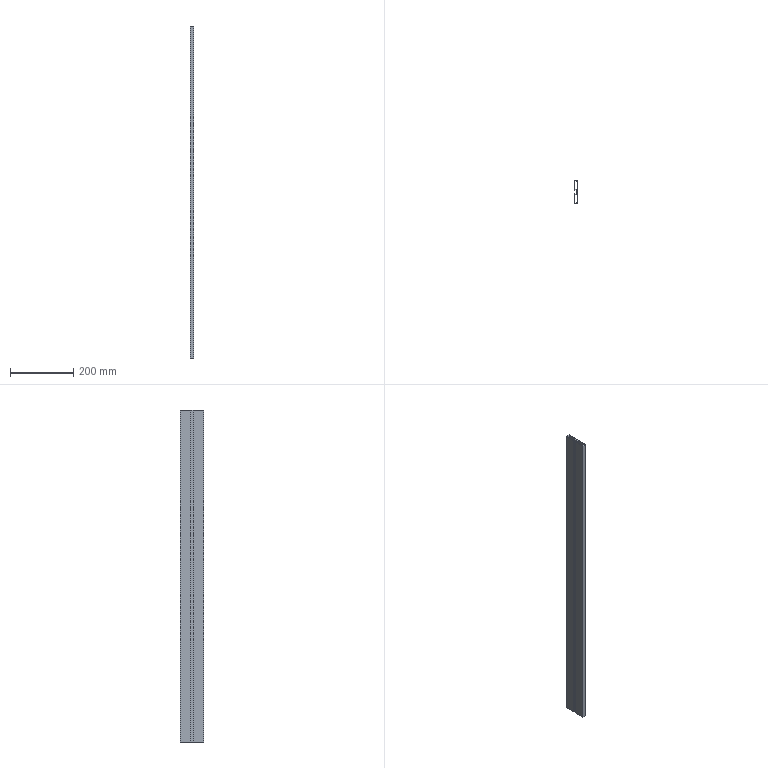Part | SolidWorks | features Extrusion 1 | 1 solid | 22 faces | box 12 x 73 x 1050 mm | volume 382200 mm3 | plane 22
STEP:
#1=CARTESIAN_POINT('',(-12.,36.5,525.));
#2=VERTEX_POINT('',#1);
#3=CARTESIAN_POINT('',(-12.,4.5,525.));
#4=VERTEX_POINT('',#3);
#5=CARTESIAN_POINT('',(-12.,36.5,525.));
#6=DIRECTION('',(0.,-1.,0.));
#7=VECTOR('',#6,1000.);
#8=LINE('',#5,#7);
#9=EDGE_CURVE('',#2,#4,#8,.T.);
#10=ORIENTED_EDGE('',*,*,#9,.T.);
#11=CARTESIAN_POINT('',(-10.,4.5,525.));
#12=VERTEX_POINT('',#11);
#13=CARTESIAN_POINT('',(-12.,4.5,525.));
#14=DIRECTION('',(1.,0.,0.));
#15=VECTOR('',#14,1000.);
#16=LINE('',#13,#15);
#17=EDGE_CURVE('',#4,#12,#16,.T.);
#18=ORIENTED_EDGE('',*,*,#17,.T.);
#19=CARTESIAN_POINT('',(-10.,6.5,525.));
#20=VERTEX_POINT('',#19);
#21=CARTESIAN_POINT('',(-10.,4.5,525.));
#22=DIRECTION('',(0.,1.,0.));
#23=VECTOR('',#22,1000.);
#24=LINE('',#21,#23);
#25=EDGE_CURVE('',#12,#20,#24,.T.);
#26=ORIENTED_EDGE('',*,*,#25,.T.);
#27=CARTESIAN_POINT('',(-4.,6.5,525.));
#28=VERTEX_POINT('',#27);
#29=CARTESIAN_POINT('',(-10.,6.5,525.));
#30=DIRECTION('',(1.,0.,0.));
#31=VECTOR('',#30,1000.);
#32=LINE('',#29,#31);
#33=EDGE_CURVE('',#20,#28,#32,.T.);
#34=ORIENTED_EDGE('',*,*,#33,.T.);
#35=CARTESIAN_POINT('',(-4.,-6.5,525.));
#36=VERTEX_POINT('',#35);
#37=CARTESIAN_POINT('',(-4.,6.5,525.));
#38=DIRECTION('',(0.,-1.,0.));
#39=VECTOR('',#38,1000.);
#40=LINE('',#37,#39);
#41=EDGE_CURVE('',#28,#36,#40,.T.);
#42=ORIENTED_EDGE('',*,*,#41,.T.);
#43=CARTESIAN_POINT('',(-10.,-6.5,525.));
#44=VERTEX_POINT('',#43);
#45=CARTESIAN_POINT('',(-4.,-6.5,525.));
#46=DIRECTION('',(-1.,0.,0.));
#47=VECTOR('',#46,1000.);
#48=LINE('',#45,#47);
#49=EDGE_CURVE('',#36,#44,#48,.T.);
#50=ORIENTED_EDGE('',*,*,#49,.T.);
#51=CARTESIAN_POINT('',(-10.,-4.5,525.));
#52=VERTEX_POINT('',#51);
#53=CARTESIAN_POINT('',(-10.,-6.5,525.));
#54=DIRECTION('',(0.,1.,0.));
#55=VECTOR('',#54,1000.);
#56=LINE('',#53,#55);
#57=EDGE_CURVE('',#44,#52,#56,.T.);
#58=ORIENTED_EDGE('',*,*,#57,.T.);
#59=CARTESIAN_POINT('',(-12.,-4.5,525.));
#60=VERTEX_POINT('',#59);
#61=CARTESIAN_POINT('',(-10.,-4.5,525.));
#62=DIRECTION('',(-1.,0.,0.));
#63=VECTOR('',#62,1000.);
#64=LINE('',#61,#63);
#65=EDGE_CURVE('',#52,#60,#64,.T.);
#66=ORIENTED_EDGE('',*,*,#65,.T.);
#67=CARTESIAN_POINT('',(-12.,-36.5,525.));
#68=VERTEX_POINT('',#67);
#69=CARTESIAN_POINT('',(-12.,-4.5,525.));
#70=DIRECTION('',(0.,-1.,0.));
#71=VECTOR('',#70,1000.);
#72=LINE('',#69,#71);
#73=EDGE_CURVE('',#60,#68,#72,.T.);
#74=ORIENTED_EDGE('',*,*,#73,.T.);
#75=CARTESIAN_POINT('',(0.,-36.5,525.));
#76=VERTEX_POINT('',#75);
#77=CARTESIAN_POINT('',(-12.,-36.5,525.));
#78=DIRECTION('',(1.,0.,0.));
#79=VECTOR('',#78,1000.);
#80=LINE('',#77,#79);
#81=EDGE_CURVE('',#68,#76,#80,.T.);
#82=ORIENTED_EDGE('',*,*,#81,.T.);
#83=CARTESIAN_POINT('',(0.,36.5,525.));
#84=VERTEX_POINT('',#83);
#85=CARTESIAN_POINT('',(0.,-36.5,525.));
#86=DIRECTION('',(0.,1.,0.));
#87=VECTOR('',#86,1000.);
#88=LINE('',#85,#87);
#89=EDGE_CURVE('',#76,#84,#88,.T.);
#90=ORIENTED_EDGE('',*,*,#89,.T.);
#91=CARTESIAN_POINT('',(0.,36.5,525.));
#92=DIRECTION('',(-1.,0.,0.));
#93=VECTOR('',#92,1000.);
#94=LINE('',#91,#93);
#95=EDGE_CURVE('',#84,#2,#94,.T.);
#96=ORIENTED_EDGE('',*,*,#95,.T.);
#97=EDGE_LOOP('',(#10,#18,#26,#34,#42,#50,#58,#66,#74,#82,#90,#96));
#98=FACE_OUTER_BOUND('',#97,.T.);
#99=CARTESIAN_POINT('',(-10.,-34.5,525.));
#100=VERTEX_POINT('',#99);
#101=CARTESIAN_POINT('',(-2.,-34.5,525.));
#102=VERTEX_POINT('',#101);
#103=CARTESIAN_POINT('',(-2.,-34.5,525.));
#104=DIRECTION('',(1.,0.,0.));
#105=VECTOR('',#104,1000.);
#106=LINE('',#103,#105);
#107=EDGE_CURVE('',#100,#102,#106,.T.);
#108=ORIENTED_EDGE('',*,*,#107,.F.);
#109=CARTESIAN_POINT('',(-10.,-8.5,525.));
#110=VERTEX_POINT('',#109);
#111=CARTESIAN_POINT('',(-10.,-34.5,525.));
#112=DIRECTION('',(0.,-1.,0.));
#113=VECTOR('',#112,1000.);
#114=LINE('',#111,#113);
#115=EDGE_CURVE('',#110,#100,#114,.T.);
#116=ORIENTED_EDGE('',*,*,#115,.F.);
#117=CARTESIAN_POINT('',(-2.,-8.5,525.));
#118=VERTEX_POINT('',#117);
#119=CARTESIAN_POINT('',(-10.,-8.5,525.));
#120=DIRECTION('',(-1.,0.,0.));
#121=VECTOR('',#120,1000.);
#122=LINE('',#119,#121);
#123=EDGE_CURVE('',#118,#110,#122,.T.);
#124=ORIENTED_EDGE('',*,*,#123,.F.);
#125=CARTESIAN_POINT('',(-2.,-8.5,525.));
#126=DIRECTION('',(0.,1.,0.));
#127=VECTOR('',#126,1000.);
#128=LINE('',#125,#127);
#129=EDGE_CURVE('',#102,#118,#128,.T.);
#130=ORIENTED_EDGE('',*,*,#129,.F.);
#131=EDGE_LOOP('',(#108,#116,#124,#130));
#132=FACE_BOUND('',#131,.T.);
#133=CARTESIAN_POINT('',(-10.,34.5,525.));
#134=VERTEX_POINT('',#133);
#135=CARTESIAN_POINT('',(-10.,8.5,525.));
#136=VERTEX_POINT('',#135);
#137=CARTESIAN_POINT('',(-10.,8.5,525.));
#138=DIRECTION('',(0.,-1.,0.));
#139=VECTOR('',#138,1000.);
#140=LINE('',#137,#139);
#141=EDGE_CURVE('',#134,#136,#140,.T.);
#142=ORIENTED_EDGE('',*,*,#141,.F.);
#143=CARTESIAN_POINT('',(-2.,34.5,525.));
#144=VERTEX_POINT('',#143);
#145=CARTESIAN_POINT('',(-10.,34.5,525.));
#146=DIRECTION('',(-1.,0.,0.));
#147=VECTOR('',#146,1000.);
#148=LINE('',#145,#147);
#149=EDGE_CURVE('',#144,#134,#148,.T.);
#150=ORIENTED_EDGE('',*,*,#149,.F.);
#151=CARTESIAN_POINT('',(-2.,8.5,525.));
#152=VERTEX_POINT('',#151);
#153=CARTESIAN_POINT('',(-2.,34.5,525.));
#154=DIRECTION('',(0.,1.,0.));
#155=VECTOR('',#154,1000.);
#156=LINE('',#153,#155);
#157=EDGE_CURVE('',#152,#144,#156,.T.);
#158=ORIENTED_EDGE('',*,*,#157,.F.);
#159=CARTESIAN_POINT('',(-2.,8.5,525.));
#160=DIRECTION('',(1.,0.,0.));
#161=VECTOR('',#160,1000.);
#162=LINE('',#159,#161);
#163=EDGE_CURVE('',#136,#152,#162,.T.);
#164=ORIENTED_EDGE('',*,*,#163,.F.);
#165=EDGE_LOOP('',(#142,#150,#158,#164));
#166=FACE_BOUND('',#165,.T.);
#167=CARTESIAN_POINT('',(0.,0.,525.));
#168=DIRECTION('',(0.,0.,1.));
#169=DIRECTION('',(1.,0.,0.));
#170=AXIS2_PLACEMENT_3D('',#167,#168,#169);
#171=PLANE('',#170);
#172=ADVANCED_FACE('',(#98,#132,#166),#171,.T.);
#173=CARTESIAN_POINT('',(-10.,-8.5,-525.));
#174=VERTEX_POINT('',#173);
#175=CARTESIAN_POINT('',(-10.,-34.5,-525.));
#176=VERTEX_POINT('',#175);
#177=CARTESIAN_POINT('',(-10.,-34.5,-525.));
#178=DIRECTION('',(0.,-1.,0.));
#179=VECTOR('',#178,1000.);
#180=LINE('',#177,#179);
#181=EDGE_CURVE('',#174,#176,#180,.T.);
#182=ORIENTED_EDGE('',*,*,#181,.T.);
#183=CARTESIAN_POINT('',(-2.,-34.5,-525.));
#184=VERTEX_POINT('',#183);
#185=CARTESIAN_POINT('',(-2.,-34.5,-525.));
#186=DIRECTION('',(1.,0.,0.));
#187=VECTOR('',#186,1000.);
#188=LINE('',#185,#187);
#189=EDGE_CURVE('',#176,#184,#188,.T.);
#190=ORIENTED_EDGE('',*,*,#189,.T.);
#191=CARTESIAN_POINT('',(-2.,-8.5,-525.));
#192=VERTEX_POINT('',#191);
#193=CARTESIAN_POINT('',(-2.,-8.5,-525.));
#194=DIRECTION('',(0.,1.,0.));
#195=VECTOR('',#194,1000.);
#196=LINE('',#193,#195);
#197=EDGE_CURVE('',#184,#192,#196,.T.);
#198=ORIENTED_EDGE('',*,*,#197,.T.);
#199=CARTESIAN_POINT('',(-10.,-8.5,-525.));
#200=DIRECTION('',(-1.,0.,0.));
#201=VECTOR('',#200,1000.);
#202=LINE('',#199,#201);
#203=EDGE_CURVE('',#192,#174,#202,.T.);
#204=ORIENTED_EDGE('',*,*,#203,.T.);
#205=EDGE_LOOP('',(#182,#190,#198,#204));
#206=FACE_BOUND('',#205,.T.);
#207=CARTESIAN_POINT('',(-12.,36.5,-525.));
#208=VERTEX_POINT('',#207);
#209=CARTESIAN_POINT('',(-12.,4.5,-525.));
#210=VERTEX_POINT('',#209);
#211=CARTESIAN_POINT('',(-12.,36.5,-525.));
#212=DIRECTION('',(0.,-1.,0.));
#213=VECTOR('',#212,1000.);
#214=LINE('',#211,#213);
#215=EDGE_CURVE('',#208,#210,#214,.T.);
#216=ORIENTED_EDGE('',*,*,#215,.F.);
#217=CARTESIAN_POINT('',(0.,36.5,-525.));
#218=VERTEX_POINT('',#217);
#219=CARTESIAN_POINT('',(0.,36.5,-525.));
#220=DIRECTION('',(-1.,0.,0.));
#221=VECTOR('',#220,1000.);
#222=LINE('',#219,#221);
#223=EDGE_CURVE('',#218,#208,#222,.T.);
#224=ORIENTED_EDGE('',*,*,#223,.F.);
#225=CARTESIAN_POINT('',(0.,-36.5,-525.));
#226=VERTEX_POINT('',#225);
#227=CARTESIAN_POINT('',(0.,-36.5,-525.));
#228=DIRECTION('',(0.,1.,0.));
#229=VECTOR('',#228,1000.);
#230=LINE('',#227,#229);
#231=EDGE_CURVE('',#226,#218,#230,.T.);
#232=ORIENTED_EDGE('',*,*,#231,.F.);
#233=CARTESIAN_POINT('',(-12.,-36.5,-525.));
#234=VERTEX_POINT('',#233);
#235=CARTESIAN_POINT('',(-12.,-36.5,-525.));
#236=DIRECTION('',(1.,0.,0.));
#237=VECTOR('',#236,1000.);
#238=LINE('',#235,#237);
#239=EDGE_CURVE('',#234,#226,#238,.T.);
#240=ORIENTED_EDGE('',*,*,#239,.F.);
#241=CARTESIAN_POINT('',(-12.,-4.5,-525.));
#242=VERTEX_POINT('',#241);
#243=CARTESIAN_POINT('',(-12.,-4.5,-525.));
#244=DIRECTION('',(0.,-1.,0.));
#245=VECTOR('',#244,1000.);
#246=LINE('',#243,#245);
#247=EDGE_CURVE('',#242,#234,#246,.T.);
#248=ORIENTED_EDGE('',*,*,#247,.F.);
#249=CARTESIAN_POINT('',(-10.,-4.5,-525.));
#250=VERTEX_POINT('',#249);
#251=CARTESIAN_POINT('',(-10.,-4.5,-525.));
#252=DIRECTION('',(-1.,0.,0.));
#253=VECTOR('',#252,1000.);
#254=LINE('',#251,#253);
#255=EDGE_CURVE('',#250,#242,#254,.T.);
#256=ORIENTED_EDGE('',*,*,#255,.F.);
#257=CARTESIAN_POINT('',(-10.,-6.5,-525.));
#258=VERTEX_POINT('',#257);
#259=CARTESIAN_POINT('',(-10.,-6.5,-525.));
#260=DIRECTION('',(0.,1.,0.));
#261=VECTOR('',#260,1000.);
#262=LINE('',#259,#261);
#263=EDGE_CURVE('',#258,#250,#262,.T.);
#264=ORIENTED_EDGE('',*,*,#263,.F.);
#265=CARTESIAN_POINT('',(-4.,-6.5,-525.));
#266=VERTEX_POINT('',#265);
#267=CARTESIAN_POINT('',(-4.,-6.5,-525.));
#268=DIRECTION('',(-1.,0.,0.));
#269=VECTOR('',#268,1000.);
#270=LINE('',#267,#269);
#271=EDGE_CURVE('',#266,#258,#270,.T.);
#272=ORIENTED_EDGE('',*,*,#271,.F.);
#273=CARTESIAN_POINT('',(-4.,6.5,-525.));
#274=VERTEX_POINT('',#273);
#275=CARTESIAN_POINT('',(-4.,6.5,-525.));
#276=DIRECTION('',(0.,-1.,0.));
#277=VECTOR('',#276,1000.);
#278=LINE('',#275,#277);
#279=EDGE_CURVE('',#274,#266,#278,.T.);
#280=ORIENTED_EDGE('',*,*,#279,.F.);
#281=CARTESIAN_POINT('',(-10.,6.5,-525.));
#282=VERTEX_POINT('',#281);
#283=CARTESIAN_POINT('',(-10.,6.5,-525.));
#284=DIRECTION('',(1.,0.,0.));
#285=VECTOR('',#284,1000.);
#286=LINE('',#283,#285);
#287=EDGE_CURVE('',#282,#274,#286,.T.);
#288=ORIENTED_EDGE('',*,*,#287,.F.);
#289=CARTESIAN_POINT('',(-10.,4.5,-525.));
#290=VERTEX_POINT('',#289);
#291=CARTESIAN_POINT('',(-10.,4.5,-525.));
#292=DIRECTION('',(0.,1.,0.));
#293=VECTOR('',#292,1000.);
#294=LINE('',#291,#293);
#295=EDGE_CURVE('',#290,#282,#294,.T.);
#296=ORIENTED_EDGE('',*,*,#295,.F.);
#297=CARTESIAN_POINT('',(-12.,4.5,-525.));
#298=DIRECTION('',(1.,0.,0.));
#299=VECTOR('',#298,1000.);
#300=LINE('',#297,#299);
#301=EDGE_CURVE('',#210,#290,#300,.T.);
#302=ORIENTED_EDGE('',*,*,#301,.F.);
#303=EDGE_LOOP('',(#216,#224,#232,#240,#248,#256,#264,#272,#280,#288,#296,#302));
#304=FACE_OUTER_BOUND('',#303,.T.);
#305=CARTESIAN_POINT('',(-2.,34.5,-525.));
#306=VERTEX_POINT('',#305);
#307=CARTESIAN_POINT('',(-10.,34.5,-525.));
#308=VERTEX_POINT('',#307);
#309=CARTESIAN_POINT('',(-10.,34.5,-525.));
#310=DIRECTION('',(-1.,0.,0.));
#311=VECTOR('',#310,1000.);
#312=LINE('',#309,#311);
#313=EDGE_CURVE('',#306,#308,#312,.T.);
#314=ORIENTED_EDGE('',*,*,#313,.T.);
#315=CARTESIAN_POINT('',(-10.,8.5,-525.));
#316=VERTEX_POINT('',#315);
#317=CARTESIAN_POINT('',(-10.,8.5,-525.));
#318=DIRECTION('',(0.,-1.,0.));
#319=VECTOR('',#318,1000.);
#320=LINE('',#317,#319);
#321=EDGE_CURVE('',#308,#316,#320,.T.);
#322=ORIENTED_EDGE('',*,*,#321,.T.);
#323=CARTESIAN_POINT('',(-2.,8.5,-525.));
#324=VERTEX_POINT('',#323);
#325=CARTESIAN_POINT('',(-2.,8.5,-525.));
#326=DIRECTION('',(1.,0.,0.));
#327=VECTOR('',#326,1000.);
#328=LINE('',#325,#327);
#329=EDGE_CURVE('',#316,#324,#328,.T.);
#330=ORIENTED_EDGE('',*,*,#329,.T.);
#331=CARTESIAN_POINT('',(-2.,34.5,-525.));
#332=DIRECTION('',(0.,1.,0.));
#333=VECTOR('',#332,1000.);
#334=LINE('',#331,#333);
#335=EDGE_CURVE('',#324,#306,#334,.T.);
#336=ORIENTED_EDGE('',*,*,#335,.T.);
#337=EDGE_LOOP('',(#314,#322,#330,#336));
#338=FACE_BOUND('',#337,.T.);
#339=CARTESIAN_POINT('',(0.,0.,-525.));
#340=DIRECTION('',(0.,0.,1.));
#341=DIRECTION('',(1.,0.,0.));
#342=AXIS2_PLACEMENT_3D('',#339,#340,#341);
#343=PLANE('',#342);
#344=ADVANCED_FACE('',(#206,#304,#338),#343,.F.);
#345=ORIENTED_EDGE('',*,*,#215,.T.);
#346=CARTESIAN_POINT('',(-12.,4.5,525.));
#347=DIRECTION('',(0.,0.,-1.));
#348=VECTOR('',#347,1000.);
#349=LINE('',#346,#348);
#350=EDGE_CURVE('',#4,#210,#349,.T.);
#351=ORIENTED_EDGE('',*,*,#350,.F.);
#352=ORIENTED_EDGE('',*,*,#9,.F.);
#353=CARTESIAN_POINT('',(-12.,36.5,525.));
#354=DIRECTION('',(0.,0.,-1.));
#355=VECTOR('',#354,1000.);
#356=LINE('',#353,#355);
#357=EDGE_CURVE('',#2,#208,#356,.T.);
#358=ORIENTED_EDGE('',*,*,#357,.T.);
#359=EDGE_LOOP('',(#345,#351,#352,#358));
#360=FACE_OUTER_BOUND('',#359,.T.);
#361=CARTESIAN_POINT('',(-12.,36.5,525.));
#362=DIRECTION('',(1.,0.,0.));
#363=DIRECTION('',(0.,0.,-1.));
#364=AXIS2_PLACEMENT_3D('',#361,#362,#363);
#365=PLANE('',#364);
#366=ADVANCED_FACE('',(#360),#365,.F.);
#367=ORIENTED_EDGE('',*,*,#301,.T.);
#368=CARTESIAN_POINT('',(-10.,4.5,525.));
#369=DIRECTION('',(0.,0.,-1.));
#370=VECTOR('',#369,1000.);
#371=LINE('',#368,#370);
#372=EDGE_CURVE('',#12,#290,#371,.T.);
#373=ORIENTED_EDGE('',*,*,#372,.F.);
#374=ORIENTED_EDGE('',*,*,#17,.F.);
#375=ORIENTED_EDGE('',*,*,#350,.T.);
#376=EDGE_LOOP('',(#367,#373,#374,#375));
#377=FACE_OUTER_BOUND('',#376,.T.);
#378=CARTESIAN_POINT('',(-12.,4.5,525.));
#379=DIRECTION('',(0.,1.,0.));
#380=DIRECTION('',(0.,0.,1.));
#381=AXIS2_PLACEMENT_3D('',#378,#379,#380);
#382=PLANE('',#381);
#383=ADVANCED_FACE('',(#377),#382,.F.);
#384=ORIENTED_EDGE('',*,*,#295,.T.);
#385=CARTESIAN_POINT('',(-10.,6.5,525.));
#386=DIRECTION('',(0.,0.,-1.));
#387=VECTOR('',#386,1000.);
#388=LINE('',#385,#387);
#389=EDGE_CURVE('',#20,#282,#388,.T.);
#390=ORIENTED_EDGE('',*,*,#389,.F.);
#391=ORIENTED_EDGE('',*,*,#25,.F.);
#392=ORIENTED_EDGE('',*,*,#372,.T.);
#393=EDGE_LOOP('',(#384,#390,#391,#392));
#394=FACE_OUTER_BOUND('',#393,.T.);
#395=CARTESIAN_POINT('',(-10.,4.5,525.));
#396=DIRECTION('',(-1.,0.,0.));
#397=DIRECTION('',(0.,0.,1.));
#398=AXIS2_PLACEMENT_3D('',#395,#396,#397);
#399=PLANE('',#398);
#400=ADVANCED_FACE('',(#394),#399,.F.);
#401=ORIENTED_EDGE('',*,*,#287,.T.);
#402=CARTESIAN_POINT('',(-4.,6.5,525.));
#403=DIRECTION('',(0.,0.,-1.));
#404=VECTOR('',#403,1000.);
#405=LINE('',#402,#404);
#406=EDGE_CURVE('',#28,#274,#405,.T.);
#407=ORIENTED_EDGE('',*,*,#406,.F.);
#408=ORIENTED_EDGE('',*,*,#33,.F.);
#409=ORIENTED_EDGE('',*,*,#389,.T.);
#410=EDGE_LOOP('',(#401,#407,#408,#409));
#411=FACE_OUTER_BOUND('',#410,.T.);
#412=CARTESIAN_POINT('',(-10.,6.5,525.));
#413=DIRECTION('',(0.,1.,0.));
#414=DIRECTION('',(0.,0.,1.));
#415=AXIS2_PLACEMENT_3D('',#412,#413,#414);
#416=PLANE('',#415);
#417=ADVANCED_FACE('',(#411),#416,.F.);
#418=ORIENTED_EDGE('',*,*,#279,.T.);
#419=CARTESIAN_POINT('',(-4.,-6.5,525.));
#420=DIRECTION('',(0.,0.,-1.));
#421=VECTOR('',#420,1000.);
#422=LINE('',#419,#421);
#423=EDGE_CURVE('',#36,#266,#422,.T.);
#424=ORIENTED_EDGE('',*,*,#423,.F.);
#425=ORIENTED_EDGE('',*,*,#41,.F.);
#426=ORIENTED_EDGE('',*,*,#406,.T.);
#427=EDGE_LOOP('',(#418,#424,#425,#426));
#428=FACE_OUTER_BOUND('',#427,.T.);
#429=CARTESIAN_POINT('',(-4.,6.5,525.));
#430=DIRECTION('',(1.,0.,0.));
#431=DIRECTION('',(0.,0.,-1.));
#432=AXIS2_PLACEMENT_3D('',#429,#430,#431);
#433=PLANE('',#432);
#434=ADVANCED_FACE('',(#428),#433,.F.);
#435=ORIENTED_EDGE('',*,*,#271,.T.);
#436=CARTESIAN_POINT('',(-10.,-6.5,525.));
#437=DIRECTION('',(0.,0.,-1.));
#438=VECTOR('',#437,1000.);
#439=LINE('',#436,#438);
#440=EDGE_CURVE('',#44,#258,#439,.T.);
#441=ORIENTED_EDGE('',*,*,#440,.F.);
#442=ORIENTED_EDGE('',*,*,#49,.F.);
#443=ORIENTED_EDGE('',*,*,#423,.T.);
#444=EDGE_LOOP('',(#435,#441,#442,#443));
#445=FACE_OUTER_BOUND('',#444,.T.);
#446=CARTESIAN_POINT('',(-4.,-6.5,525.));
#447=DIRECTION('',(0.,-1.,0.));
#448=DIRECTION('',(0.,0.,-1.));
#449=AXIS2_PLACEMENT_3D('',#446,#447,#448);
#450=PLANE('',#449);
#451=ADVANCED_FACE('',(#445),#450,.F.);
#452=ORIENTED_EDGE('',*,*,#263,.T.);
#453=CARTESIAN_POINT('',(-10.,-4.5,525.));
#454=DIRECTION('',(0.,0.,-1.));
#455=VECTOR('',#454,1000.);
#456=LINE('',#453,#455);
#457=EDGE_CURVE('',#52,#250,#456,.T.);
#458=ORIENTED_EDGE('',*,*,#457,.F.);
#459=ORIENTED_EDGE('',*,*,#57,.F.);
#460=ORIENTED_EDGE('',*,*,#440,.T.);
#461=EDGE_LOOP('',(#452,#458,#459,#460));
#462=FACE_OUTER_BOUND('',#461,.T.);
#463=CARTESIAN_POINT('',(-10.,-6.5,525.));
#464=DIRECTION('',(-1.,0.,0.));
#465=DIRECTION('',(0.,0.,1.));
#466=AXIS2_PLACEMENT_3D('',#463,#464,#465);
#467=PLANE('',#466);
#468=ADVANCED_FACE('',(#462),#467,.F.);
#469=ORIENTED_EDGE('',*,*,#255,.T.);
#470=CARTESIAN_POINT('',(-12.,-4.5,525.));
#471=DIRECTION('',(0.,0.,-1.));
#472=VECTOR('',#471,1000.);
#473=LINE('',#470,#472);
#474=EDGE_CURVE('',#60,#242,#473,.T.);
#475=ORIENTED_EDGE('',*,*,#474,.F.);
#476=ORIENTED_EDGE('',*,*,#65,.F.);
#477=ORIENTED_EDGE('',*,*,#457,.T.);
#478=EDGE_LOOP('',(#469,#475,#476,#477));
#479=FACE_OUTER_BOUND('',#478,.T.);
#480=CARTESIAN_POINT('',(-10.,-4.5,525.));
#481=DIRECTION('',(0.,-1.,0.));
#482=DIRECTION('',(0.,0.,-1.));
#483=AXIS2_PLACEMENT_3D('',#480,#481,#482);
#484=PLANE('',#483);
#485=ADVANCED_FACE('',(#479),#484,.F.);
#486=ORIENTED_EDGE('',*,*,#247,.T.);
#487=CARTESIAN_POINT('',(-12.,-36.5,525.));
#488=DIRECTION('',(0.,0.,-1.));
#489=VECTOR('',#488,1000.);
#490=LINE('',#487,#489);
#491=EDGE_CURVE('',#68,#234,#490,.T.);
#492=ORIENTED_EDGE('',*,*,#491,.F.);
#493=ORIENTED_EDGE('',*,*,#73,.F.);
#494=ORIENTED_EDGE('',*,*,#474,.T.);
#495=EDGE_LOOP('',(#486,#492,#493,#494));
#496=FACE_OUTER_BOUND('',#495,.T.);
#497=CARTESIAN_POINT('',(-12.,-4.5,525.));
#498=DIRECTION('',(1.,0.,0.));
#499=DIRECTION('',(0.,0.,-1.));
#500=AXIS2_PLACEMENT_3D('',#497,#498,#499);
#501=PLANE('',#500);
#502=ADVANCED_FACE('',(#496),#501,.F.);
#503=ORIENTED_EDGE('',*,*,#239,.T.);
#504=CARTESIAN_POINT('',(0.,-36.5,525.));
#505=DIRECTION('',(0.,0.,-1.));
#506=VECTOR('',#505,1000.);
#507=LINE('',#504,#506);
#508=EDGE_CURVE('',#76,#226,#507,.T.);
#509=ORIENTED_EDGE('',*,*,#508,.F.);
#510=ORIENTED_EDGE('',*,*,#81,.F.);
#511=ORIENTED_EDGE('',*,*,#491,.T.);
#512=EDGE_LOOP('',(#503,#509,#510,#511));
#513=FACE_OUTER_BOUND('',#512,.T.);
#514=CARTESIAN_POINT('',(-12.,-36.5,525.));
#515=DIRECTION('',(0.,1.,0.));
#516=DIRECTION('',(0.,0.,1.));
#517=AXIS2_PLACEMENT_3D('',#514,#515,#516);
#518=PLANE('',#517);
#519=ADVANCED_FACE('',(#513),#518,.F.);
#520=ORIENTED_EDGE('',*,*,#231,.T.);
#521=CARTESIAN_POINT('',(0.,36.5,525.));
#522=DIRECTION('',(0.,0.,-1.));
#523=VECTOR('',#522,1000.);
#524=LINE('',#521,#523);
#525=EDGE_CURVE('',#84,#218,#524,.T.);
#526=ORIENTED_EDGE('',*,*,#525,.F.);
#527=ORIENTED_EDGE('',*,*,#89,.F.);
#528=ORIENTED_EDGE('',*,*,#508,.T.);
#529=EDGE_LOOP('',(#520,#526,#527,#528));
#530=FACE_OUTER_BOUND('',#529,.T.);
#531=CARTESIAN_POINT('',(0.,-36.5,525.));
#532=DIRECTION('',(-1.,0.,0.));
#533=DIRECTION('',(0.,0.,1.));
#534=AXIS2_PLACEMENT_3D('',#531,#532,#533);
#535=PLANE('',#534);
#536=ADVANCED_FACE('',(#530),#535,.F.);
#537=ORIENTED_EDGE('',*,*,#223,.T.);
#538=ORIENTED_EDGE('',*,*,#357,.F.);
#539=ORIENTED_EDGE('',*,*,#95,.F.);
#540=ORIENTED_EDGE('',*,*,#525,.T.);
#541=EDGE_LOOP('',(#537,#538,#539,#540));
#542=FACE_OUTER_BOUND('',#541,.T.);
#543=CARTESIAN_POINT('',(0.,36.5,525.));
#544=DIRECTION('',(0.,-1.,0.));
#545=DIRECTION('',(0.,0.,-1.));
#546=AXIS2_PLACEMENT_3D('',#543,#544,#545);
#547=PLANE('',#546);
#548=ADVANCED_FACE('',(#542),#547,.F.);
#549=ORIENTED_EDGE('',*,*,#181,.F.);
#550=CARTESIAN_POINT('',(-10.,-8.5,525.));
#551=DIRECTION('',(0.,0.,-1.));
#552=VECTOR('',#551,1000.);
#553=LINE('',#550,#552);
#554=EDGE_CURVE('',#110,#174,#553,.T.);
#555=ORIENTED_EDGE('',*,*,#554,.F.);
#556=ORIENTED_EDGE('',*,*,#115,.T.);
#557=CARTESIAN_POINT('',(-10.,-34.5,525.));
#558=DIRECTION('',(0.,0.,-1.));
#559=VECTOR('',#558,1000.);
#560=LINE('',#557,#559);
#561=EDGE_CURVE('',#100,#176,#560,.T.);
#562=ORIENTED_EDGE('',*,*,#561,.T.);
#563=EDGE_LOOP('',(#549,#555,#556,#562));
#564=FACE_OUTER_BOUND('',#563,.T.);
#565=CARTESIAN_POINT('',(-10.,-34.5,525.));
#566=DIRECTION('',(1.,0.,0.));
#567=DIRECTION('',(0.,0.,-1.));
#568=AXIS2_PLACEMENT_3D('',#565,#566,#567);
#569=PLANE('',#568);
#570=ADVANCED_FACE('',(#564),#569,.T.);
#571=ORIENTED_EDGE('',*,*,#189,.F.);
#572=ORIENTED_EDGE('',*,*,#561,.F.);
#573=ORIENTED_EDGE('',*,*,#107,.T.);
#574=CARTESIAN_POINT('',(-2.,-34.5,525.));
#575=DIRECTION('',(0.,0.,-1.));
#576=VECTOR('',#575,1000.);
#577=LINE('',#574,#576);
#578=EDGE_CURVE('',#102,#184,#577,.T.);
#579=ORIENTED_EDGE('',*,*,#578,.T.);
#580=EDGE_LOOP('',(#571,#572,#573,#579));
#581=FACE_OUTER_BOUND('',#580,.T.);
#582=CARTESIAN_POINT('',(-2.,-34.5,525.));
#583=DIRECTION('',(0.,1.,0.));
#584=DIRECTION('',(0.,0.,1.));
#585=AXIS2_PLACEMENT_3D('',#582,#583,#584);
#586=PLANE('',#585);
#587=ADVANCED_FACE('',(#581),#586,.T.);
#588=ORIENTED_EDGE('',*,*,#197,.F.);
#589=ORIENTED_EDGE('',*,*,#578,.F.);
#590=ORIENTED_EDGE('',*,*,#129,.T.);
#591=CARTESIAN_POINT('',(-2.,-8.5,525.));
#592=DIRECTION('',(0.,0.,-1.));
#593=VECTOR('',#592,1000.);
#594=LINE('',#591,#593);
#595=EDGE_CURVE('',#118,#192,#594,.T.);
#596=ORIENTED_EDGE('',*,*,#595,.T.);
#597=EDGE_LOOP('',(#588,#589,#590,#596));
#598=FACE_OUTER_BOUND('',#597,.T.);
#599=CARTESIAN_POINT('',(-2.,-8.5,525.));
#600=DIRECTION('',(-1.,0.,0.));
#601=DIRECTION('',(0.,0.,1.));
#602=AXIS2_PLACEMENT_3D('',#599,#600,#601);
#603=PLANE('',#602);
#604=ADVANCED_FACE('',(#598),#603,.T.);
#605=ORIENTED_EDGE('',*,*,#203,.F.);
#606=ORIENTED_EDGE('',*,*,#595,.F.);
#607=ORIENTED_EDGE('',*,*,#123,.T.);
#608=ORIENTED_EDGE('',*,*,#554,.T.);
#609=EDGE_LOOP('',(#605,#606,#607,#608));
#610=FACE_OUTER_BOUND('',#609,.T.);
#611=CARTESIAN_POINT('',(-10.,-8.5,525.));
#612=DIRECTION('',(0.,-1.,0.));
#613=DIRECTION('',(0.,0.,-1.));
#614=AXIS2_PLACEMENT_3D('',#611,#612,#613);
#615=PLANE('',#614);
#616=ADVANCED_FACE('',(#610),#615,.T.);
#617=ORIENTED_EDGE('',*,*,#313,.F.);
#618=CARTESIAN_POINT('',(-2.,34.5,525.));
#619=DIRECTION('',(0.,0.,-1.));
#620=VECTOR('',#619,1000.);
#621=LINE('',#618,#620);
#622=EDGE_CURVE('',#144,#306,#621,.T.);
#623=ORIENTED_EDGE('',*,*,#622,.F.);
#624=ORIENTED_EDGE('',*,*,#149,.T.);
#625=CARTESIAN_POINT('',(-10.,34.5,525.));
#626=DIRECTION('',(0.,0.,-1.));
#627=VECTOR('',#626,1000.);
#628=LINE('',#625,#627);
#629=EDGE_CURVE('',#134,#308,#628,.T.);
#630=ORIENTED_EDGE('',*,*,#629,.T.);
#631=EDGE_LOOP('',(#617,#623,#624,#630));
#632=FACE_OUTER_BOUND('',#631,.T.);
#633=CARTESIAN_POINT('',(-10.,34.5,525.));
#634=DIRECTION('',(0.,-1.,0.));
#635=DIRECTION('',(0.,0.,-1.));
#636=AXIS2_PLACEMENT_3D('',#633,#634,#635);
#637=PLANE('',#636);
#638=ADVANCED_FACE('',(#632),#637,.T.);
#639=ORIENTED_EDGE('',*,*,#321,.F.);
#640=ORIENTED_EDGE('',*,*,#629,.F.);
#641=ORIENTED_EDGE('',*,*,#141,.T.);
#642=CARTESIAN_POINT('',(-10.,8.5,525.));
#643=DIRECTION('',(0.,0.,-1.));
#644=VECTOR('',#643,1000.);
#645=LINE('',#642,#644);
#646=EDGE_CURVE('',#136,#316,#645,.T.);
#647=ORIENTED_EDGE('',*,*,#646,.T.);
#648=EDGE_LOOP('',(#639,#640,#641,#647));
#649=FACE_OUTER_BOUND('',#648,.T.);
#650=CARTESIAN_POINT('',(-10.,8.5,525.));
#651=DIRECTION('',(1.,0.,0.));
#652=DIRECTION('',(0.,0.,-1.));
#653=AXIS2_PLACEMENT_3D('',#650,#651,#652);
#654=PLANE('',#653);
#655=ADVANCED_FACE('',(#649),#654,.T.);
#656=ORIENTED_EDGE('',*,*,#329,.F.);
#657=ORIENTED_EDGE('',*,*,#646,.F.);
#658=ORIENTED_EDGE('',*,*,#163,.T.);
#659=CARTESIAN_POINT('',(-2.,8.5,525.));
#660=DIRECTION('',(0.,0.,-1.));
#661=VECTOR('',#660,1000.);
#662=LINE('',#659,#661);
#663=EDGE_CURVE('',#152,#324,#662,.T.);
#664=ORIENTED_EDGE('',*,*,#663,.T.);
#665=EDGE_LOOP('',(#656,#657,#658,#664));
#666=FACE_OUTER_BOUND('',#665,.T.);
#667=CARTESIAN_POINT('',(-2.,8.5,525.));
#668=DIRECTION('',(0.,1.,0.));
#669=DIRECTION('',(0.,0.,1.));
#670=AXIS2_PLACEMENT_3D('',#667,#668,#669);
#671=PLANE('',#670);
#672=ADVANCED_FACE('',(#666),#671,.T.);
#673=ORIENTED_EDGE('',*,*,#335,.F.);
#674=ORIENTED_EDGE('',*,*,#663,.F.);
#675=ORIENTED_EDGE('',*,*,#157,.T.);
#676=ORIENTED_EDGE('',*,*,#622,.T.);
#677=EDGE_LOOP('',(#673,#674,#675,#676));
#678=FACE_OUTER_BOUND('',#677,.T.);
#679=CARTESIAN_POINT('',(-2.,34.5,525.));
#680=DIRECTION('',(-1.,0.,0.));
#681=DIRECTION('',(0.,0.,1.));
#682=AXIS2_PLACEMENT_3D('',#679,#680,#681);
#683=PLANE('',#682);
#684=ADVANCED_FACE('',(#678),#683,.T.);
#685=CLOSED_SHELL('',(#172,#344,#366,#383,#400,#417,#434,#451,#468,#485,#502,#519,#536,#548,#570,#587,#604,#616,#638,#655,#672,#684));
#686=MANIFOLD_SOLID_BREP('',#685);
#687=CARTESIAN_POINT('',(0.,0.,0.));
#688=DIRECTION('',(0.,0.,1.));
#689=DIRECTION('',(1.,0.,0.));
#690=AXIS2_PLACEMENT_3D('',#687,#688,#689);
#691=(LENGTH_UNIT()NAMED_UNIT(*)SI_UNIT(.MILLI.,.METRE.));
#692=UNCERTAINTY_MEASURE_WITH_UNIT(LENGTH_MEASURE(0.00001),#691,'','');
#693=(NAMED_UNIT(*)PLANE_ANGLE_UNIT()SI_UNIT($,.RADIAN.));
#694=(NAMED_UNIT(*)SI_UNIT($,.STERADIAN.)SOLID_ANGLE_UNIT());
#695=(GEOMETRIC_REPRESENTATION_CONTEXT(3)GLOBAL_UNCERTAINTY_ASSIGNED_CONTEXT((#692))GLOBAL_UNIT_ASSIGNED_CONTEXT((#691,#693,#694))REPRESENTATION_CONTEXT('',''));
#696=ADVANCED_BREP_SHAPE_REPRESENTATION('',(#686,#690),#695);